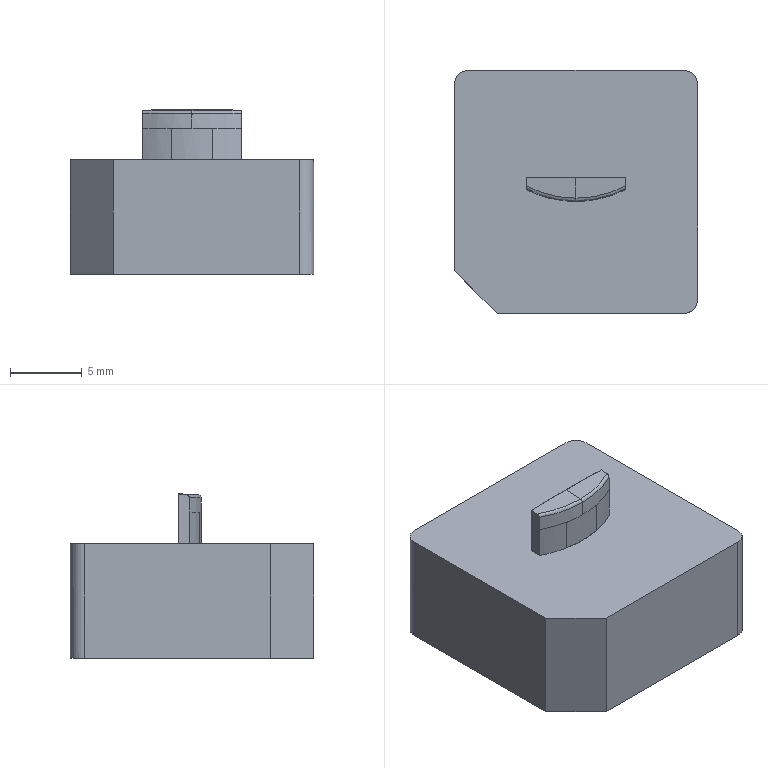NC program | PowerMill | posted with a generic post | part box 17 x 17 x 11.498 mm
Lines 11660 to 12582 of 31087:
N11757 M6
N11758 S18000 M03
N11759 G00 G90 X0.0 Y0.0
N11760 G43 Z10.798 H10
N11761
N11762 G05 P10000 R8
N11763 X-0.5869 Y2.8775
N11764 Z1.0084
N11765 G01 Z-0.1916 F1200.0
N11766 X-0.5849 Y2.8338 F2000.0
N11767 X-0.5789 Y2.7904
N11768 X-0.569 Y2.7478
N11769 X-0.5553 Y2.7063
N11770 X-0.5378 Y2.6661
N11771 X-0.5168 Y2.6277
N11772 X-0.4923 Y2.5915
N11773 X-0.4647 Y2.5575
N11774 X-0.4341 Y2.5263
N11775 X-0.4007 Y2.498
N11776 X-0.365 Y2.4728
N11777 X-0.327 Y2.451
N11778 X-0.2872 Y2.4327
N11779 X-0.246 Y2.4181
N11780 X-0.2036 Y2.4073
N11781 X-0.1604 Y2.4005
N11782 X-0.1167 Y2.3976
N11783 X-0.1069 Y2.3975
N11784 X2.2486
N11785 X3.0991 Y2.3979
N11786 X3.1754 Y2.3965
N11787 X3.2515 Y2.3917
N11788 X3.3271 Y2.3832
N11789 X3.4006 Y2.371
N11790 X3.4718 Y2.3554
N11791 X3.5409 Y2.3365
N11792 X3.6082 Y2.3147
N11793 X3.6742 Y2.2895
N11794 X3.7407 Y2.2599
N11795 X3.8074 Y2.226
N11796 X3.8734 Y2.188
N11797 X3.9376 Y2.1464
N11798 X3.9988 Y2.1021
N11799 X4.0562 Y2.0557
N11800 X4.1001 Y2.0167
N11801 X4.1422 Y1.9756
N11802 X4.1829 Y1.9321
N11803 X4.2295 Y1.8782
N11804 X4.2752 Y1.8201
N11805 X4.3115 Y1.7694
N11806 X4.3434 Y1.7201
N11807 X4.3726 Y1.6691
N11808 X4.4032 Y1.6099
N11809 X4.4345 Y1.5427
N11810 X4.4641 Y1.4704
N11811 X4.4886 Y1.4011
N11812 X4.5077 Y1.3368
N11813 X4.5228 Y1.2731
N11814 X4.5369 Y1.1976
N11815 X4.5469 Y1.1222
N11816 X4.5529 Y1.0471
N11817 X4.5549 Y0.9725
N11818 X4.5529 Y0.8986
N11819 X4.547 Y0.8253
N11820 X4.5396 Y0.7669
N11821 X4.5303 Y0.7089
N11822 X4.5185 Y0.6513
N11823 X4.5036 Y0.5944
N11824 X4.4867 Y0.538
N11825 X4.4703 Y0.4871
N11826 X4.4513 Y0.4371
N11827 X4.4263 Y0.3814
N11828 X4.3917 Y0.3126
N11829 X4.3587 Y0.2521
N11830 X4.3215 Y0.192
N11831 X4.2798 Y0.1319
N11832 X4.2334 Y0.0721
N11833 X4.1823 Y0.0126
N11834 X4.1341 Y-0.0382
N11835 X4.0821 Y-0.0874
N11836 X4.0258 Y-0.1351
N11837 X3.9666 Y-0.1804
N11838 X3.9063 Y-0.2222
N11839 X3.8444 Y-0.2607
N11840 X3.7808 Y-0.2957
N11841 X3.7158 Y-0.3271
N11842 X3.6494 Y-0.3547
N11843 X3.5818 Y-0.3787
N11844 X3.5128 Y-0.3994
N11845 X3.442 Y-0.4174
N11846 X3.3467 Y-0.438
N11847 X3.2184 Y-0.4626
N11848 X3.0991 Y-0.4856
N11849 X2.9555 Y-0.5129
N11850 X2.7831 Y-0.5421
N11851 X2.5349 Y-0.5811
N11852 X2.4186 Y-0.5998
N11853 X2.351 Y-0.6099
N11854 X2.2832 Y-0.6191
N11855 X2.2154 Y-0.628
N11856 X2.1475 Y-0.6366
N11857 X2.0605 Y-0.6476
N11858 X1.9926 Y-0.656
N11859 X1.9247 Y-0.6643
N11860 X1.8568 Y-0.6726
N11861 X1.7889 Y-0.6808
N11862 X1.694 Y-0.6903
N11863 X1.5848 Y-0.6998
N11864 X1.4547 Y-0.7118
N11865 X1.3245 Y-0.7235
N11866 X1.1943 Y-0.7338
N11867 X1.0639 Y-0.7416
N11868 X0.9334 Y-0.7483
N11869 X0.6647 Y-0.7625
N11870 X0.5541 Y-0.7674
N11871 X0.4308 Y-0.7699
N11872 X0.3025 Y-0.771
N11873 X0.1586 Y-0.7742
N11874 X0.0315 Y-0.7766
N11875 X-0.0497 Y-0.7759
N11876 X-0.1534 Y-0.7721
N11877 X-0.2619 Y-0.769
N11878 X-0.4707 Y-0.7657
N11879 X-0.5531 Y-0.7642
N11880 X-0.6356 Y-0.7611
N11881 X-0.718 Y-0.7574
N11882 X-0.8004 Y-0.7534
N11883 X-0.89 Y-0.7486
N11884 X-0.9724 Y-0.7439
N11885 X-1.0547 Y-0.7391
N11886 X-1.1371 Y-0.734
N11887 X-1.2194 Y-0.7285
N11888 X-1.3017 Y-0.7227
N11889 X-1.3839 Y-0.7157
N11890 X-1.5706 Y-0.6989
N11891 X-1.7572 Y-0.681
N11892 X-1.9435 Y-0.6606
N11893 X-2.1295 Y-0.6376
N11894 X-2.3152 Y-0.6126
N11895 X-2.5033 Y-0.5862
N11896 X-2.691 Y-0.5576
N11897 X-2.8782 Y-0.5253
N11898 X-2.9988 Y-0.5037
N11899 X-3.1948 Y-0.4681
N11900 X-3.3381 Y-0.4397
N11901 X-3.4588 Y-0.4126
N11902 X-3.5132 Y-0.3991
N11903 X-3.5672 Y-0.3839
N11904 X-3.6205 Y-0.3664
N11905 X-3.6727 Y-0.3461
N11906 X-3.729 Y-0.3208
N11907 X-3.7835 Y-0.2928
N11908 X-3.8325 Y-0.2652
N11909 X-3.8809 Y-0.2365
N11910 X-3.9285 Y-0.2068
N11911 X-3.9829 Y-0.1688
N11912 X-4.0363 Y-0.1266
N11913 X-4.0884 Y-0.0805
N11914 X-4.1295 Y-0.0409
N11915 X-4.1699 Y-0.0006
N11916 X-4.2085 Y0.0413
N11917 X-4.2447 Y0.0855
N11918 X-4.2786 Y0.1314
N11919 X-4.3115 Y0.1781
N11920 X-4.3414 Y0.2219
N11921 X-4.3686 Y0.2674
N11922 X-4.3969 Y0.3218
N11923 X-4.432 Y0.3958
N11924 X-4.458 Y0.4556
N11925 X-4.4815 Y0.5192
N11926 X-4.5022 Y0.5864
N11927 X-4.5198 Y0.6569
N11928 X-4.5342 Y0.7301
N11929 X-4.5449 Y0.8055
N11930 X-4.5517 Y0.8821
N11931 X-4.5546 Y0.9588
N11932 X-4.5535 Y1.0343
N11933 X-4.5486 Y1.1081
N11934 X-4.54 Y1.1795
N11935 X-4.528 Y1.2488
N11936 X-4.5124 Y1.3182
N11937 X-4.4931 Y1.3873
N11938 X-4.4699 Y1.4565
N11939 X-4.4424 Y1.5257
N11940 X-4.4107 Y1.5951
N11941 X-4.3749 Y1.6642
N11942 X-4.3438 Y1.7188
N11943 X-4.3098 Y1.7717
N11944 X-4.2726 Y1.8236
N11945 X-4.2289 Y1.879
N11946 X-4.1787 Y1.9366
N11947 X-4.1258 Y1.9916
N11948 X-4.0741 Y2.0402
N11949 X-4.0249 Y2.082
N11950 X-3.9749 Y2.1202
N11951 X-3.9118 Y2.1639
N11952 X-3.8469 Y2.2039
N11953 X-3.7805 Y2.2402
N11954 X-3.7127 Y2.2727
N11955 X-3.6438 Y2.3014
N11956 X-3.5773 Y2.3251
N11957 X-3.5102 Y2.3455
N11958 X-3.4413 Y2.3627
N11959 X-3.3699 Y2.3766
N11960 X-3.2959 Y2.387
N11961 X-3.2193 Y2.3938
N11962 X-3.1417 Y2.3971
N11963 X-3.063 Y2.3975
N11964 X-0.1069
N11965 X-0.0632 Y2.3995
N11966 X-0.0198 Y2.4055
N11967 X0.0228 Y2.4153
N11968 X0.0644 Y2.4291
N11969 X0.1045 Y2.4465
N11970 X0.1429 Y2.4676
N11971 X0.1792 Y2.492
N11972 X0.2131 Y2.5197
N11973 X0.2443 Y2.5503
N11974 X0.2727 Y2.5836
N11975 X0.2978 Y2.6194
N11976 X0.3197 Y2.6573
N11977 X0.3379 Y2.6971
N11978 X0.3525 Y2.7384
N11979 X0.3633 Y2.7808
N11980 X0.3701 Y2.824
N11981 X0.373 Y2.8676
N11982 X0.3731 Y2.8775
N11983 X-0.5869 Y2.8776 Z-0.2215
N11984 X-0.5849 Y2.8339
N11985 X-0.5789 Y2.7906
N11986 X-0.569 Y2.748
N11987 X-0.5553 Y2.7064
N11988 X-0.5378 Y2.6663
N11989 X-0.5168 Y2.6279
N11990 X-0.4923 Y2.5916
N11991 X-0.4647 Y2.5577
N11992 X-0.4341 Y2.5264
N11993 X-0.4007 Y2.4981
N11994 X-0.365 Y2.4729
N11995 X-0.327 Y2.4511
N11996 X-0.2873 Y2.4328
N11997 X-0.246 Y2.4182
N11998 X-0.2036 Y2.4075
N11999 X-0.1604 Y2.4006
N12000 X-0.1167 Y2.3977
N12001 X-0.1069 Y2.3976
N12002 X1.6447 Y2.3977
N12003 X3.3145 Y2.3985
N12004 X3.399 Y2.3986
N12005 X3.483 Y2.3971
N12006 X3.5641 Y2.3922
N12007 X3.6423 Y2.384
N12008 X3.7177 Y2.3722
N12009 X3.7906 Y2.357
N12010 X3.8612 Y2.3382
N12011 X3.9297 Y2.316
N12012 X3.9964 Y2.2905
N12013 X4.0622 Y2.2613
N12014 X4.1298 Y2.227
N12015 X4.1955 Y2.1893
N12016 X4.2591 Y2.1481
N12017 X4.3204 Y2.1037
N12018 X4.3793 Y2.056
N12019 X4.4356 Y2.0054
N12020 X4.4893 Y1.9518
N12021 X4.5398 Y1.8957
N12022 X4.587 Y1.8374
N12023 X4.6307 Y1.7771
N12024 X4.6709 Y1.715
N12025 X4.7074 Y1.6512
N12026 X4.7402 Y1.5859
N12027 X4.7718 Y1.5145
N12028 X4.7987 Y1.4443
N12029 X4.8211 Y1.3752
N12030 X4.8393 Y1.3069
N12031 X4.8511 Y1.2526
N12032 X4.8611 Y1.1979
N12033 X4.8689 Y1.143
N12034 X4.8744 Y1.0877
N12035 X4.8781 Y1.023
N12036 X4.8794 Y0.9544
N12037 Y0.8986
N12038 X4.8792 Y0.8428
N12039 X4.8791 Y0.7871
N12040 Y0.5998
N12041 X4.8776 Y0.5049
N12042 X4.8732 Y0.4225
N12043 X4.8657 Y0.3482
N12044 X4.8556 Y0.281
N12045 X4.8417 Y0.2135
N12046 X4.8232 Y0.1436
N12047 X4.8001 Y0.0711
N12048 X4.774 Y0.0018
N12049 X4.744 Y-0.0667
N12050 X4.7101 Y-0.1341
N12051 X4.6726 Y-0.1999
N12052 X4.6321 Y-0.263
N12053 X4.5882 Y-0.324
N12054 X4.5412 Y-0.3826
N12055 X4.491 Y-0.4387
N12056 X4.4379 Y-0.4921
N12057 X4.3819 Y-0.5428
N12058 X4.3233 Y-0.5904
N12059 X4.2623 Y-0.6348
N12060 X4.1992 Y-0.6758
N12061 X4.134 Y-0.7135
N12062 X4.067 Y-0.7475
N12063 X3.9988 Y-0.7778
N12064 X3.9496 Y-0.7972
N12065 X3.8998 Y-0.8149
N12066 X3.8493 Y-0.8306
N12067 X3.7902 Y-0.8463
N12068 X3.7301 Y-0.86
N12069 X3.6781 Y-0.8709
N12070 X3.626 Y-0.8815
N12071 X3.5741 Y-0.8923
N12072 X3.5222 Y-0.9034
N12073 X3.3732 Y-0.935
N12074 X3.2238 Y-0.9643
N12075 X3.0738 Y-0.9906
N12076 X2.9235 Y-1.0154
N12077 X2.7484 Y-1.0439
N12078 X2.5732 Y-1.0714
N12079 X2.3991 Y-1.0967
N12080 X2.3212 Y-1.107
N12081 X2.2432 Y-1.1169
N12082 X2.1651 Y-1.1266
N12083 X2.0854 Y-1.1363
N12084 X1.9675 Y-1.1502
N12085 X1.8894 Y-1.1591
N12086 X1.8112 Y-1.1678
N12087 X1.733 Y-1.176
N12088 X1.6548 Y-1.1835
N12089 X1.6274 Y-1.1857
N12090 X1.4698 Y-1.1989
N12091 X1.2905 Y-1.2145
N12092 X1.1492 Y-1.2244
N12093 X0.9235 Y-1.2378
N12094 X0.6977 Y-1.2487
N12095 X0.4879 Y-1.2557
N12096 X0.278 Y-1.2599
N12097 X0.0681 Y-1.2627
N12098 X-0.0156 Y-1.2636
N12099 X-0.0993 Y-1.2633
N12100 X-0.183 Y-1.2621
N12101 X-0.2667 Y-1.2605
N12102 X-0.3601 Y-1.2584
N12103 X-0.4438 Y-1.2563
N12104 X-0.5275 Y-1.254
N12105 X-0.6111 Y-1.2515
N12106 X-0.6948 Y-1.2486
N12107 X-0.7785 Y-1.245
N12108 X-1.0383 Y-1.232
N12109 X-1.263 Y-1.2176
N12110 X-1.3686 Y-1.2091
N12111 X-1.4874 Y-1.1983
N12112 X-1.5931 Y-1.1898
N12113 X-1.7169 Y-1.1793
N12114 X-1.8406 Y-1.1674
N12115 X-1.964 Y-1.1534
N12116 X-2.0873 Y-1.1378
N12117 X-2.2106 Y-1.1219
N12118 X-2.3339 Y-1.1064
N12119 X-2.4572 Y-1.0906
N12120 X-2.5955 Y-1.0699
N12121 X-2.7923 Y-1.0374
N12122 X-2.8992 Y-1.0201
N12123 X-3.0249 Y-0.9998
N12124 X-3.128 Y-0.9805
N12125 X-3.2344 Y-0.9605
N12126 X-3.341 Y-0.9411
N12127 X-3.4473 Y-0.9203
N12128 X-3.5532 Y-0.8976
N12129 X-3.6004 Y-0.887
N12130 X-3.6478 Y-0.8766
N12131 X-3.6953 Y-0.8667
N12132 X-3.7446 Y-0.8563
N12133 X-3.8083 Y-0.8417
N12134 X-3.855 Y-0.829
N12135 X-3.901 Y-0.8145
N12136 X-3.9465 Y-0.7981
N12137 X-3.9913 Y-0.78
N12138 X-4.0358 Y-0.7607
N12139 X-4.0897 Y-0.7363
N12140 X-4.1426 Y-0.7097
N12141 X-4.1937 Y-0.6798
N12142 X-4.243 Y-0.6472
N12143 X-4.2914 Y-0.6131
N12144 X-4.3389 Y-0.5778
N12145 X-4.3947 Y-0.5319
N12146 X-4.4483 Y-0.4825
N12147 X-4.4998 Y-0.4297
N12148 X-4.5488 Y-0.3738
N12149 X-4.5952 Y-0.3147
N12150 X-4.6388 Y-0.2528
N12151 X-4.6795 Y-0.1883
N12152 X-4.716 Y-0.1229
N12153 X-4.7492 Y-0.0554
N12154 X-4.7789 Y0.0141
N12155 X-4.805 Y0.0851
N12156 X-4.8271 Y0.1571
N12157 X-4.8453 Y0.2298
N12158 X-4.8596 Y0.3028
N12159 X-4.8697 Y0.3757
N12160 X-4.8759 Y0.4483
N12161 X-4.8782 Y0.5204
N12162 X-4.8797 Y0.7031
N12163 X-4.8791 Y0.8859
N12164 X-4.878 Y0.9997
N12165 X-4.8751 Y1.0736
N12166 X-4.8682 Y1.1473
N12167 X-4.8574 Y1.2208
N12168 X-4.8426 Y1.2938
N12169 X-4.8238 Y1.3662
N12170 X-4.8011 Y1.4378
N12171 X-4.7746 Y1.5083
N12172 X-4.7443 Y1.5775
N12173 X-4.7103 Y1.6452
N12174 X-4.673 Y1.7107
N12175 X-4.6323 Y1.774
N12176 X-4.5883 Y1.8352
N12177 X-4.5411 Y1.8939
N12178 X-4.4908 Y1.9501
N12179 X-4.4377 Y2.0036
N12180 X-4.3817 Y2.0542
N12181 X-4.3232 Y2.1018
N12182 X-4.2623 Y2.1461
N12183 X-4.1991 Y2.1872
N12184 X-4.1339 Y2.2248
N12185 X-4.0668 Y2.259
N12186 X-3.9979 Y2.2895
N12187 X-3.9313 Y2.315
N12188 X-3.8635 Y2.3371
N12189 X-3.7937 Y2.3559
N12190 X-3.7216 Y2.3714
N12191 X-3.6467 Y2.3834
N12192 X-3.5686 Y2.3919
N12193 X-3.4873 Y2.397
N12194 X-3.4024 Y2.3986
N12195 X-3.3155 Y2.3985
N12196 X-1.6749 Y2.3976
N12197 X-0.1069
N12198 X-0.0632 Y2.3996
N12199 X-0.0198 Y2.4056
N12200 X0.0228 Y2.4155
N12201 X0.0644 Y2.4292
N12202 X0.1045 Y2.4467
N12203 X0.1429 Y2.4677
N12204 X0.1792 Y2.4922
N12205 X0.2131 Y2.5198
N12206 X0.2443 Y2.5505
N12207 X0.2727 Y2.5838
N12208 X0.2978 Y2.6196
N12209 X0.3197 Y2.6575
N12210 X0.3379 Y2.6973
N12211 X0.3525 Y2.7385
N12212 X0.3633 Y2.7809
N12213 X0.3701 Y2.8241
N12214 X0.373 Y2.8678
N12215 X0.3731 Y2.8776
N12216 G00 Z2.9492
N12217 G01 X2.1865 Y-2.1012 F10000.0
N12218 G00 Z0.9485
N12219 G01 Z-0.2515 F1200.0
N12220 X2.1809 Y-2.0578 F2000.0
N12221 X2.1713 Y-2.0151
N12222 X2.1579 Y-1.9734
N12223 X2.1408 Y-1.9332
N12224 X2.1201 Y-1.8946
N12225 X2.0959 Y-1.8581
N12226 X2.0685 Y-1.824
N12227 X2.0382 Y-1.7925
N12228 X2.0051 Y-1.7639
N12229 X1.9695 Y-1.7384
N12230 X1.9318 Y-1.7163
N12231 X1.8922 Y-1.6977
N12232 X1.851 Y-1.6828
N12233 X1.8087 Y-1.6717
N12234 X1.7655 Y-1.6645
N12235 X1.7219 Y-1.6612
N12236 X1.6782 Y-1.662
N12237 X1.6683 Y-1.6627
N12238 X1.4407 Y-1.6816
N12239 X1.2128 Y-1.6983
N12240 X0.9848 Y-1.7118
N12241 X0.7566 Y-1.7221
N12242 X0.5654 Y-1.7289
N12243 X0.3741 Y-1.734
N12244 X0.1828 Y-1.7366
N12245 X0.0 Y-1.7377
N12246 X-0.1468 Y-1.7367
N12247 X-0.3656 Y-1.7329
N12248 X-0.5295 Y-1.7299
N12249 X-0.7199 Y-1.723
N12250 X-0.8714 Y-1.7161
N12251 X-1.0229 Y-1.7091
N12252 X-1.1743 Y-1.7006
N12253 X-1.3146 Y-1.6905
N12254 X-1.4549 Y-1.68
N12255 X-1.5953 Y-1.6693
N12256 X-1.7355 Y-1.6573
N12257 X-1.8754 Y-1.6432
N12258 X-1.9993 Y-1.6286
N12259 X-2.111 Y-1.6126
N12260 X-2.2297 Y-1.5918
N12261 X-2.3571 Y-1.5655
N12262 X-2.4967 Y-1.5328
N12263 X-2.6544 Y-1.4928
N12264 X-2.7993 Y-1.4535
N12265 X-2.8824 Y-1.4284
N12266 X-2.9933 Y-1.3931
N12267 X-3.0999 Y-1.3592
N12268 X-3.2412 Y-1.3107
N12269 X-3.3988 Y-1.2526
N12270 X-3.586 Y-1.1798
N12271 X-3.7066 Y-1.1304
N12272 X-3.8525 Y-1.0669
N12273 X-4.0025 Y-1.0
N12274 X-4.0756 Y-0.9656
N12275 X-4.1456 Y-0.9284
N12276 X-4.2126 Y-0.8885
N12277 X-4.2764 Y-0.8459
N12278 X-4.3372 Y-0.8006
N12279 X-4.3951 Y-0.7527
N12280 X-4.4499 Y-0.7021
N12281 X-4.5018 Y-0.6487
N12282 X-4.5508 Y-0.5928
N12283 X-4.5968 Y-0.5342
N12284 X-4.6399 Y-0.4729
N12285 X-4.6802 Y-0.4089
N12286 X-4.7169 Y-0.3434
N12287 X-4.7497 Y-0.2768
N12288 X-4.7786 Y-0.2094
N12289 X-4.8034 Y-0.1413
N12290 X-4.8264 Y-0.0669
N12291 X-4.8452 Y0.0069
N12292 X-4.8597 Y0.0799
N12293 X-4.8702 Y0.152
N12294 X-4.8765 Y0.2229
N12295 X-4.8789 Y0.2927
N12296 Y0.3624
N12297 X-4.8788 Y0.9997
N12298 X-4.8768 Y1.065
N12299 X-4.8709 Y1.1325
N12300 X-4.8608 Y1.2024
N12301 X-4.8463 Y1.2752
N12302 X-4.8273 Y1.3512
N12303 X-4.807 Y1.4195
N12304 X-4.783 Y1.4869
N12305 X-4.7549 Y1.5545
N12306 X-4.7225 Y1.6219
N12307 X-4.6865 Y1.6878
N12308 X-4.6471 Y1.752
N12309 X-4.6043 Y1.8139
N12310 X-4.5583 Y1.8734
N12311 X-4.5092 Y1.9305
N12312 X-4.4571 Y1.9849
N12313 X-4.4021 Y2.0365
N12314 X-4.3445 Y2.0851
N12315 X-4.2844 Y2.1307
N12316 X-4.2219 Y2.173
N12317 X-4.1573 Y2.2118
N12318 X-4.0909 Y2.2473
N12319 X-4.0226 Y2.2791
N12320 X-3.9565 Y2.3059
N12321 X-3.8897 Y2.3291
N12322 X-3.8209 Y2.3492
N12323 X-3.7498 Y2.3659
N12324 X-3.6761 Y2.3792
N12325 X-3.5993 Y2.389
N12326 X-3.5192 Y2.3954
N12327 X-3.4354 Y2.3983
N12328 X-3.3485 Y2.3985
N12329 X-1.6892 Y2.3976
N12330 X1.6447 Y2.3977
N12331 X3.3149 Y2.3985
N12332 X3.399 Y2.3986
N12333 X3.483 Y2.3971
N12334 X3.5641 Y2.3922
N12335 X3.6423 Y2.384
N12336 X3.7177 Y2.3722
N12337 X3.7906 Y2.357
N12338 X3.8612 Y2.3382
N12339 X3.9297 Y2.316
N12340 X3.9964 Y2.2905
N12341 X4.0622 Y2.2613
N12342 X4.1298 Y2.227
N12343 X4.1955 Y2.1893
N12344 X4.2591 Y2.1481
N12345 X4.3204 Y2.1037
N12346 X4.3793 Y2.056
N12347 X4.4356 Y2.0054
N12348 X4.4893 Y1.9518
N12349 X4.5398 Y1.8957
N12350 X4.587 Y1.8374
N12351 X4.6307 Y1.7771
N12352 X4.6709 Y1.715
N12353 X4.7074 Y1.6512
N12354 X4.7402 Y1.5859
N12355 X4.7717 Y1.5145
N12356 X4.7988 Y1.4439
N12357 X4.8214 Y1.3739
N12358 X4.8398 Y1.3046
N12359 X4.8526 Y1.247
N12360 X4.8644 Y1.1826
N12361 X4.871 Y1.1305
N12362 X4.8743 Y1.0814
N12363 X4.8778 Y0.9818
N12364 X4.879 Y0.8822
N12365 X4.8791 Y0.7826
N12366 X4.8792 Y0.4981
N12367 X4.8791 Y0.3999
N12368 X4.8784 Y0.3127
N12369 X4.876 Y0.2256
N12370 X4.8718 Y0.162
N12371 X4.8638 Y0.0974
N12372 X4.8516 Y0.0306
N12373 X4.8349 Y-0.0389
N12374 X4.8136 Y-0.1113
N12375 X4.7884 Y-0.1837
N12376 X4.7602 Y-0.2534
N12377 X4.7289 Y-0.3202
N12378 X4.6946 Y-0.3842
N12379 X4.6549 Y-0.45
N12380 X4.6131 Y-0.512
N12381 X4.5691 Y-0.5702
N12382 X4.5228 Y-0.6251
N12383 X4.4745 Y-0.6771
N12384 X4.4237 Y-0.7268
N12385 X4.3702 Y-0.7741
N12386 X4.3136 Y-0.8192
N12387 X4.2536 Y-0.862
N12388 X4.1898 Y-0.9026
N12389 X4.1219 Y-0.9412
N12390 X4.0498 Y-0.9778
N12391 X3.9774 Y-1.0109
N12392 X3.8384 Y-1.0726
N12393 X3.6988 Y-1.133
N12394 X3.5583 Y-1.191
N12395 X3.4166 Y-1.2461
N12396 X3.2737 Y-1.2991
N12397 X3.1297 Y-1.3492
N12398 X2.999 Y-1.3916
N12399 X2.8874 Y-1.4263
N12400 X2.7753 Y-1.4596
N12401 X2.6626 Y-1.4906
N12402 X2.5496 Y-1.5205
N12403 X2.4995 Y-1.5337
N12404 X2.4577 Y-1.5438
N12405 X2.4156 Y-1.5529
N12406 X2.3735 Y-1.5617
N12407 X2.3268 Y-1.5711
N12408 X2.2639 Y-1.5834
N12409 X2.1906 Y-1.5973
N12410 X2.1394 Y-1.6066
N12411 X2.097 Y-1.6141
N12412 X2.0546 Y-1.6212
N12413 X2.012 Y-1.6277
N12414 X1.9693 Y-1.6328
N12415 X1.7955 Y-1.6511
N12416 X1.6683 Y-1.6627
N12417 X1.3788 Y-1.6886 Z-0.2516
N12418 X1.152 Y-1.7062 Z-0.2518
N12419 X0.952 Y-1.7185 Z-0.2519
N12420 X0.7358 Y-1.7303 Z-0.252
N12421 X0.5196 Y-1.7406 Z-0.2521
N12422 X0.3032 Y-1.7471 Z-0.2523
N12423 X0.0867 Y-1.7511 Z-0.2524
N12424 X-0.0505 Y-1.7531 Z-0.2525
N12425 X-0.2019 Y-1.7524 Z-0.2526
N12426 X-0.407 Y-1.7498 Z-0.2527
N12427 X-0.5453 Y-1.7484
N12428 X-0.7071 Y-1.7436 Z-0.2528
N12429 X-0.851 Y-1.738
N12430 X-1.0867 Y-1.7268 Z-0.2529
N12431 X-1.3243 Y-1.7116
N12432 X-1.5461 Y-1.6939 Z-0.2528
N12433 X-1.7809 Y-1.6716
N12434 X-1.894 Y-1.6603 Z-0.2529
N12435 X-1.9933 Y-1.6483 Z-0.2532
N12436 X-2.1019 Y-1.6315 Z-0.2535
N12437 X-2.2252 Y-1.6086 Z-0.254
N12438 X-2.3769 Y-1.5769 Z-0.2547
N12439 X-2.4914 Y-1.5508 Z-0.2552
N12440 X-2.6248 Y-1.517 Z-0.2559
N12441 X-2.7746 Y-1.4769 Z-0.2567
N12442 X-2.8686 Y-1.4511 Z-0.2571
N12443 X-2.9722 Y-1.4191 Z-0.2573
N12444 X-3.103 Y-1.3751 Z-0.2575
N12445 X-3.293 Y-1.3082 Z-0.2577
N12446 X-3.4555 Y-1.2477 Z-0.2579
N12447 X-3.6005 Y-1.19 Z-0.2581
N12448 X-3.7419 Y-1.1305 Z-0.2583
N12449 X-3.9023 Y-1.0602 Z-0.2585
N12450 X-4.0413 Y-0.9958 Z-0.2587
N12451 X-4.1078 Y-0.9634 Z-0.2588
N12452 X-4.1729 Y-0.928 Z-0.2589
N12453 X-4.2361 Y-0.8892 Z-0.259
N12454 X-4.2975 Y-0.8468 Z-0.2591
N12455 X-4.3567 Y-0.8011 Z-0.2592
N12456 X-4.4136 Y-0.7521 Z-0.2593
N12457 X-4.4681 Y-0.6999 Z-0.2594
N12458 X-4.5198 Y-0.6448
N12459 X-4.5683 Y-0.5874 Z-0.2595
N12460 X-4.6137 Y-0.5275 Z-0.2596
N12461 X-4.656 Y-0.4652 Z-0.2597
N12462 X-4.6948 Y-0.4007 Z-0.2598
N12463 X-4.7302 Y-0.3343 Z-0.2599
N12464 X-4.762 Y-0.2661 Z-0.26
N12465 X-4.7901 Y-0.1962 Z-0.2601
N12466 X-4.8145 Y-0.1249 Z-0.2602
N12467 X-4.8351 Y-0.0525 Z-0.2603
N12468 X-4.8519 Y0.0209 Z-0.2604
N12469 X-4.8647 Y0.095 Z-0.2605
N12470 X-4.8735 Y0.1698 Z-0.2606
N12471 X-4.8784 Y0.2448 Z-0.2607
N12472 X-4.8794 Y0.3201
N12473 X-4.8788 Y0.9997 Z-0.2616
N12474 X-4.8768 Y1.0633 Z-0.2617
N12475 X-4.8713 Y1.127
N12476 X-4.8619 Y1.1952 Z-0.2618
N12477 X-4.8482 Y1.2673 Z-0.2619
N12478 X-4.8302 Y1.3419 Z-0.262
N12479 X-4.8084 Y1.4158 Z-0.2621
N12480 X-4.7837 Y1.4858 Z-0.2622
N12481 X-4.757 Y1.5507 Z-0.2623
N12482 X-4.7286 Y1.6106 Z-0.2624
N12483 X-4.6922 Y1.6781 Z-0.2625
N12484 X-4.6525 Y1.7434 Z-0.2626
N12485 X-4.6096 Y1.8062
N12486 X-4.5637 Y1.8664 Z-0.2627
N12487 X-4.5149 Y1.9239 Z-0.2628
N12488 X-4.4634 Y1.9784 Z-0.2629
N12489 X-4.409 Y2.0302 Z-0.263
N12490 X-4.3519 Y2.079 Z-0.2631
N12491 X-4.2922 Y2.1249 Z-0.2632
N12492 X-4.23 Y2.1676 Z-0.2633
N12493 X-4.1654 Y2.2071 Z-0.2634
N12494 X-4.0986 Y2.2433 Z-0.2635
N12495 X-4.0297 Y2.2761 Z-0.2636
N12496 X-3.9648 Y2.303 Z-0.2637
N12497 X-3.8988 Y2.3266 Z-0.2638
N12498 X-3.8313 Y2.3467
N12499 X-3.7614 Y2.3637 Z-0.2639
N12500 X-3.6886 Y2.3773 Z-0.264
N12501 X-3.6125 Y2.3876 Z-0.2641
N12502 X-3.5323 Y2.3946 Z-0.2642
N12503 X-3.4472 Y2.3981 Z-0.2643
N12504 X-3.3568 Y2.3984 Z-0.2644
N12505 X-1.6508 Y2.3976 Z-0.2665
N12506 X1.6379 Z-0.2706
N12507 X3.3254 Y2.3985 Z-0.2727
N12508 X3.399 Y2.3986 Z-0.2728
N12509 X3.4832 Y2.3971 Z-0.2729
N12510 X3.5643 Y2.3922 Z-0.273
N12511 X3.6424 Y2.384 Z-0.2731
N12512 X3.7178 Y2.3723 Z-0.2732
N12513 X3.7905 Y2.3571
N12514 X3.8609 Y2.3384 Z-0.2733
N12515 X3.9292 Y2.3163 Z-0.2734
N12516 X3.9956 Y2.2908 Z-0.2735
N12517 X4.061 Y2.2617 Z-0.2736
N12518 X4.1292 Y2.2273 Z-0.2737
N12519 X4.1951 Y2.1895 Z-0.2738
N12520 X4.2586 Y2.1486 Z-0.2739
N12521 X4.3195 Y2.1046 Z-0.274
N12522 X4.3778 Y2.0576 Z-0.2741
N12523 X4.4334 Y2.0077 Z-0.2742
N12524 X4.4862 Y1.9549
N12525 X4.5368 Y1.8988 Z-0.2743
N12526 X4.5845 Y1.8399 Z-0.2744
N12527 X4.6291 Y1.7785 Z-0.2745
N12528 X4.6704 Y1.7148 Z-0.2746
N12529 X4.7085 Y1.6488 Z-0.2747
N12530 X4.7384 Y1.5905 Z-0.2748
N12531 X4.7654 Y1.5307 Z-0.2749
N12532 X4.7906 Y1.4668 Z-0.275
N12533 X4.814 Y1.3976 Z-0.2751
N12534 X4.8347 Y1.3243
N12535 X4.8518 Y1.25 Z-0.2752
N12536 X4.8646 Y1.1771 Z-0.2753
N12537 X4.8731 Y1.1068 Z-0.2754
N12538 X4.8776 Y1.0399 Z-0.2755
N12539 X4.8785 Y0.9744 Z-0.2756
N12540 X4.8795 Y0.5114 Z-0.2762
N12541 X4.8782 Y0.1986 Z-0.2765
N12542 X4.8764 Y0.1614 Z-0.2766
N12543 X4.8726 Y0.1245
N12544 X4.8673 Y0.0854 Z-0.2767
N12545 X4.8594 Y0.0371
N12546 X4.847 Y-0.0261 Z-0.2768
N12547 X4.8323 Y-0.0896 Z-0.2769
N12548 X4.8194 Y-0.1374 Z-0.277
N12549 X4.8076 Y-0.1756
N12550 X4.7952 Y-0.2107 Z-0.2771
N12551 X4.7641 Y-0.2872 Z-0.2772
N12552 X4.7314 Y-0.3581 Z-0.2773
N12553 X4.697 Y-0.424
N12554 X4.6607 Y-0.4852 Z-0.2774
N12555 X4.6216 Y-0.544 Z-0.2775
N12556 X4.5761 Y-0.6053 Z-0.2776
N12557 X4.5277 Y-0.6639 Z-0.2777
N12558 X4.4764 Y-0.7197 Z-0.2778
N12559 X4.4225 Y-0.7725 Z-0.2779
N12560 X4.366 Y-0.8223 Z-0.278
N12561 X4.3073 Y-0.8688 Z-0.2781
N12562 X4.2462 Y-0.9121 Z-0.2782
N12563 X4.1852 Y-0.9508 Z-0.2783
N12564 X4.1245 Y-0.9848
N12565 X4.063 Y-1.0156 Z-0.2784
N12566 X3.9102 Y-1.0888 Z-0.2786
N12567 X3.7558 Y-1.1588 Z-0.2788
N12568 X3.6001 Y-1.2257 Z-0.2791
N12569 X3.4433 Y-1.29 Z-0.2793
N12570 X3.2723 Y-1.3564 Z-0.2795
N12571 X3.1001 Y-1.4194 Z-0.2797
N12572 X2.9251 Y-1.4791 Z-0.2799
N12573 X2.7504 Y-1.5348 Z-0.2802
N12574 X2.5746 Y-1.5869 Z-0.2804
N12575 X2.4113 Y-1.6321 Z-0.2806
N12576 X2.2473 Y-1.6746 Z-0.2808
N12577 X2.0825 Y-1.7138 Z-0.281
N12578 X1.9169 Y-1.7497 Z-0.2812
N12579 X1.7507 Y-1.7827 Z-0.2814
N12580 X1.6915 Y-1.7939 Z-0.2815
N12581 X1.5219 Y-1.8234 Z-0.2817
N12582 X1.3353 Y-1.852 Z-0.282
N12583 X1.1647 Y-1.8752 Z-0.2822
N12584 X0.9828 Y-1.8965 Z-0.2824
N12585 X0.8006 Y-1.9141 Z-0.2826
N12586 X0.618 Y-1.9279 Z-0.2828
N12587 X0.4351 Y-1.9382 Z-0.2831
N12588 X0.2771 Y-1.9443 Z-0.2833
N12589 X0.1191 Y-1.9484 Z-0.2835
N12590 X-0.039 Y-1.9498 Z-0.2837
N12591 X-0.1971 Y-1.9478 Z-0.2838
N12592 X-0.3551 Y-1.9435 Z-0.284
N12593 X-0.543 Y-1.9351 Z-0.2843
N12594 X-0.7357 Y-1.9227 Z-0.2845
N12595 X-0.9289 Y-1.9063 Z-0.2847
N12596 X-1.1175 Y-1.8863 Z-0.285
N12597 X-1.3013 Y-1.8631 Z-0.2852
N12598 X-1.4792 Y-1.8369 Z-0.2854
N12599 X-1.6607 Y-1.8065 Z-0.2856
N12600 X-1.8471 Y-1.7715 Z-0.2859
N12601 X-2.0362 Y-1.732 Z-0.2861
N12602 X-2.2244 Y-1.6886 Z-0.2864
N12603 X-2.4084 Y-1.6423 Z-0.2866
N12604 X-2.5864 Y-1.5935 Z-0.2868
N12605 X-2.7587 Y-1.5424 Z-0.287
N12606 X-2.9237 Y-1.4897 Z-0.2872
N12607 X-3.11 Y-1.4263 Z-0.2875
N12608 X-3.2841 Y-1.3632 Z-0.2877
N12609 X-3.4482 Y-1.2997 Z-0.2879
N12610 X-3.6084 Y-1.234 Z-0.2881
N12611 X-3.7782 Y-1.161 Z-0.2884
N12612 X-3.9317 Y-1.0911 Z-0.2886
N12613 X-4.073 Y-1.023 Z-0.2888
N12614 X-4.1386 Y-0.9894 Z-0.2889
N12615 X-4.2025 Y-0.9527 Z-0.289
N12616 X-4.2646 Y-0.9124
N12617 X-4.3248 Y-0.8687 Z-0.2891
N12618 X-4.3828 Y-0.8216 Z-0.2892
N12619 X-4.4385 Y-0.7712 Z-0.2893
N12620 X-4.4917 Y-0.7178 Z-0.2894
N12621 X-4.5422 Y-0.6613 Z-0.2895
N12622 X-4.5899 Y-0.6021 Z-0.2896
N12623 X-4.6318 Y-0.5441 Z-0.2897
N12624 X-4.6715 Y-0.4824 Z-0.2898
N12625 X-4.7095 Y-0.4161 Z-0.2899
N12626 X-4.7458 Y-0.3448 Z-0.29
N12627 X-4.7677 Y-0.2975
N12628 X-4.7859 Y-0.2529 Z-0.2901
N12629 X-4.8019 Y-0.2074
N12630 X-4.8164 Y-0.1614 Z-0.2902
N12631 X-4.8316 Y-0.1069 Z-0.2903
N12632 X-4.8479 Y-0.0395 Z-0.2904
N12633 X-4.8621 Y0.0327
N12634 X-4.8712 Y0.0926 Z-0.2905
N12635 X-4.8763 Y0.1433 Z-0.2906
N12636 X-4.8786 Y0.1913
N12637 Y0.2395 Z-0.2907
N12638 X-4.8783 Y0.9997 Z-0.2916
N12639 X-4.8764 Y1.064 Z-0.2917
N12640 X-4.8708 Y1.1294 Z-0.2918
N12641 X-4.8612 Y1.1985 Z-0.2919
N12642 X-4.8474 Y1.2708 Z-0.292
N12643 X-4.8293 Y1.3449 Z-0.2921
N12644 X-4.8072 Y1.4188 Z-0.2922
N12645 X-4.7819 Y1.4895 Z-0.2923
N12646 X-4.7543 Y1.556
N12647 X-4.7246 Y1.6181 Z-0.2924
N12648 X-4.6884 Y1.6846 Z-0.2925
N12649 X-4.6488 Y1.7492 Z-0.2926
N12650 X-4.6058 Y1.8115 Z-0.2927
N12651 X-4.5595 Y1.8716 Z-0.2928
N12652 X-4.5102 Y1.929 Z-0.2929
N12653 X-4.458 Y1.9838 Z-0.293
N12654 X-4.4036 Y2.0351 Z-0.2931
N12655 X-4.3465 Y2.0834 Z-0.2932
N12656 X-4.2868 Y2.1288 Z-0.2933
N12657 X-4.2245 Y2.1712 Z-0.2934
N12658 X-4.1597 Y2.2104
N12659 X-4.0926 Y2.2463 Z-0.2935
N12660 X-4.0233 Y2.2789 Z-0.2936
N12661 X-3.9585 Y2.3055 Z-0.2937
N12662 X-3.8924 Y2.3287 Z-0.2938
N12663 X-3.8247 Y2.3485 Z-0.2939
N12664 X-3.7546 Y2.3651 Z-0.294
N12665 X-3.6816 Y2.3785 Z-0.2941
N12666 X-3.6051 Y2.3885 Z-0.2942
N12667 X-3.5245 Y2.395 Z-0.2943
N12668 X-3.4389 Y2.3982 Z-0.2944
N12669 X-3.3479 Y2.3984 Z-0.2945
N12670 X-1.6375 Y2.3976 Z-0.2966
N12671 X1.6401 Z-0.3006
N12672 X3.3265 Y2.3985 Z-0.3027
N12673 X3.399 Y2.3986 Z-0.3028
N12674 X3.4832 Y2.3971 Z-0.3029
N12675 X3.5643 Y2.3922 Z-0.303
N12676 X3.6424 Y2.384 Z-0.3031
N12677 X3.7178 Y2.3723
N12678 X3.7905 Y2.357 Z-0.3032
N12679 X3.8609 Y2.3384 Z-0.3033